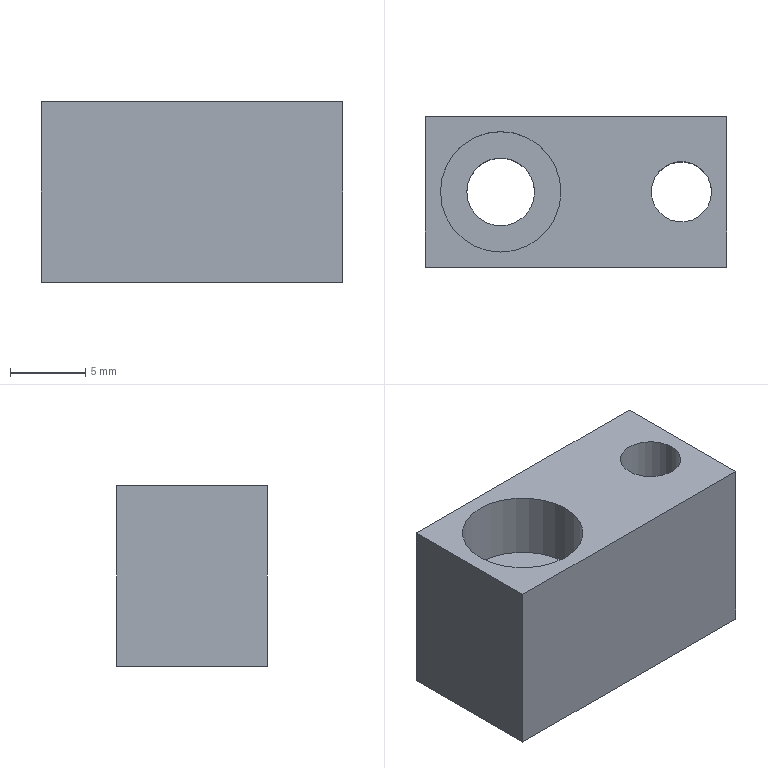Part | NX | features BREP 1 | 1 solid | 10 faces | box 20 x 10 x 12 mm | volume 1907 mm3 | plane 7 | cylinder 3 | commonest cylinder face diameters 4 x1 4.5 x1 8 x1
STEP:
#1=CARTESIAN_POINT('',(10.,-5.,0.));
#2=VERTEX_POINT('',#1);
#3=CARTESIAN_POINT('',(10.,5.,0.));
#4=VERTEX_POINT('',#3);
#5=CARTESIAN_POINT('',(10.,5.,0.));
#6=DIRECTION('',(0.,1.,0.));
#7=VECTOR('',#6,1000.);
#8=LINE('',#5,#7);
#9=EDGE_CURVE('',#2,#4,#8,.T.);
#10=ORIENTED_EDGE('',*,*,#9,.F.);
#11=CARTESIAN_POINT('',(10.,-5.,-12.));
#12=VERTEX_POINT('',#11);
#13=CARTESIAN_POINT('',(10.,-5.,-12.));
#14=DIRECTION('',(0.,0.,1.));
#15=VECTOR('',#14,1000.);
#16=LINE('',#13,#15);
#17=EDGE_CURVE('',#12,#2,#16,.T.);
#18=ORIENTED_EDGE('',*,*,#17,.F.);
#19=CARTESIAN_POINT('',(10.,5.,-12.));
#20=VERTEX_POINT('',#19);
#21=CARTESIAN_POINT('',(10.,5.,-12.));
#22=DIRECTION('',(0.,1.,0.));
#23=VECTOR('',#22,1000.);
#24=LINE('',#21,#23);
#25=EDGE_CURVE('',#12,#20,#24,.T.);
#26=ORIENTED_EDGE('',*,*,#25,.T.);
#27=CARTESIAN_POINT('',(10.,5.,-12.));
#28=DIRECTION('',(0.,0.,1.));
#29=VECTOR('',#28,1000.);
#30=LINE('',#27,#29);
#31=EDGE_CURVE('',#20,#4,#30,.T.);
#32=ORIENTED_EDGE('',*,*,#31,.T.);
#33=EDGE_LOOP('',(#10,#18,#26,#32));
#34=FACE_BOUND('',#33,.T.);
#35=CARTESIAN_POINT('',(10.,5.,-12.));
#36=DIRECTION('',(-1.,0.,0.));
#37=DIRECTION('',(0.,0.,1.));
#38=AXIS2_PLACEMENT_3D('',#35,#36,#37);
#39=PLANE('',#38);
#40=ADVANCED_FACE('',(#34),#39,.F.);
#41=CARTESIAN_POINT('',(-10.,5.,0.));
#42=VERTEX_POINT('',#41);
#43=CARTESIAN_POINT('',(-10.,5.,0.));
#44=DIRECTION('',(-1.,0.,0.));
#45=VECTOR('',#44,1000.);
#46=LINE('',#43,#45);
#47=EDGE_CURVE('',#4,#42,#46,.T.);
#48=ORIENTED_EDGE('',*,*,#47,.F.);
#49=ORIENTED_EDGE('',*,*,#31,.F.);
#50=CARTESIAN_POINT('',(-10.,5.,-12.));
#51=VERTEX_POINT('',#50);
#52=CARTESIAN_POINT('',(-10.,5.,-12.));
#53=DIRECTION('',(-1.,0.,0.));
#54=VECTOR('',#53,1000.);
#55=LINE('',#52,#54);
#56=EDGE_CURVE('',#20,#51,#55,.T.);
#57=ORIENTED_EDGE('',*,*,#56,.T.);
#58=CARTESIAN_POINT('',(-10.,5.,-12.));
#59=DIRECTION('',(0.,0.,1.));
#60=VECTOR('',#59,1000.);
#61=LINE('',#58,#60);
#62=EDGE_CURVE('',#51,#42,#61,.T.);
#63=ORIENTED_EDGE('',*,*,#62,.T.);
#64=EDGE_LOOP('',(#48,#49,#57,#63));
#65=FACE_BOUND('',#64,.T.);
#66=CARTESIAN_POINT('',(-10.,5.,-12.));
#67=DIRECTION('',(0.,-1.,0.));
#68=DIRECTION('',(0.,0.,-1.));
#69=AXIS2_PLACEMENT_3D('',#66,#67,#68);
#70=PLANE('',#69);
#71=ADVANCED_FACE('',(#65),#70,.F.);
#72=CARTESIAN_POINT('',(-10.,-5.,0.));
#73=VERTEX_POINT('',#72);
#74=CARTESIAN_POINT('',(-10.,5.,0.));
#75=DIRECTION('',(0.,-1.,0.));
#76=VECTOR('',#75,1000.);
#77=LINE('',#74,#76);
#78=EDGE_CURVE('',#42,#73,#77,.T.);
#79=ORIENTED_EDGE('',*,*,#78,.F.);
#80=ORIENTED_EDGE('',*,*,#62,.F.);
#81=CARTESIAN_POINT('',(-10.,-5.,-12.));
#82=VERTEX_POINT('',#81);
#83=CARTESIAN_POINT('',(-10.,5.,-12.));
#84=DIRECTION('',(0.,-1.,0.));
#85=VECTOR('',#84,1000.);
#86=LINE('',#83,#85);
#87=EDGE_CURVE('',#51,#82,#86,.T.);
#88=ORIENTED_EDGE('',*,*,#87,.T.);
#89=CARTESIAN_POINT('',(-10.,-5.,-12.));
#90=DIRECTION('',(0.,0.,1.));
#91=VECTOR('',#90,1000.);
#92=LINE('',#89,#91);
#93=EDGE_CURVE('',#82,#73,#92,.T.);
#94=ORIENTED_EDGE('',*,*,#93,.T.);
#95=EDGE_LOOP('',(#79,#80,#88,#94));
#96=FACE_BOUND('',#95,.T.);
#97=CARTESIAN_POINT('',(-10.,5.,-12.));
#98=DIRECTION('',(1.,0.,0.));
#99=DIRECTION('',(0.,0.,-1.));
#100=AXIS2_PLACEMENT_3D('',#97,#98,#99);
#101=PLANE('',#100);
#102=ADVANCED_FACE('',(#96),#101,.F.);
#103=CARTESIAN_POINT('',(-10.,-5.,0.));
#104=DIRECTION('',(1.,0.,0.));
#105=VECTOR('',#104,1000.);
#106=LINE('',#103,#105);
#107=EDGE_CURVE('',#73,#2,#106,.T.);
#108=ORIENTED_EDGE('',*,*,#107,.F.);
#109=ORIENTED_EDGE('',*,*,#93,.F.);
#110=CARTESIAN_POINT('',(-10.,-5.,-12.));
#111=DIRECTION('',(1.,0.,0.));
#112=VECTOR('',#111,1000.);
#113=LINE('',#110,#112);
#114=EDGE_CURVE('',#82,#12,#113,.T.);
#115=ORIENTED_EDGE('',*,*,#114,.T.);
#116=ORIENTED_EDGE('',*,*,#17,.T.);
#117=EDGE_LOOP('',(#108,#109,#115,#116));
#118=FACE_BOUND('',#117,.T.);
#119=CARTESIAN_POINT('',(-10.,-5.,-12.));
#120=DIRECTION('',(0.,1.,0.));
#121=DIRECTION('',(0.,0.,1.));
#122=AXIS2_PLACEMENT_3D('',#119,#120,#121);
#123=PLANE('',#122);
#124=ADVANCED_FACE('',(#118),#123,.F.);
#125=CARTESIAN_POINT('',(-7.25,0.,-12.));
#126=VERTEX_POINT('',#125);
#127=CARTESIAN_POINT('',(-5.,0.,-12.));
#128=DIRECTION('',(0.,0.,-1.));
#129=DIRECTION('',(-1.,0.,0.));
#130=AXIS2_PLACEMENT_3D('',#127,#128,#129);
#131=CIRCLE('',#130,2.25);
#132=EDGE_CURVE('',#126,#126,#131,.T.);
#133=ORIENTED_EDGE('',*,*,#132,.F.);
#134=EDGE_LOOP('',(#133));
#135=FACE_BOUND('',#134,.T.);
#136=CARTESIAN_POINT('',(5.,0.,-12.));
#137=VERTEX_POINT('',#136);
#138=CARTESIAN_POINT('',(7.,0.,-12.));
#139=DIRECTION('',(0.,0.,-1.));
#140=DIRECTION('',(-1.,0.,0.));
#141=AXIS2_PLACEMENT_3D('',#138,#139,#140);
#142=CIRCLE('',#141,2.);
#143=EDGE_CURVE('',#137,#137,#142,.T.);
#144=ORIENTED_EDGE('',*,*,#143,.F.);
#145=EDGE_LOOP('',(#144));
#146=FACE_BOUND('',#145,.T.);
#147=ORIENTED_EDGE('',*,*,#25,.F.);
#148=ORIENTED_EDGE('',*,*,#114,.F.);
#149=ORIENTED_EDGE('',*,*,#87,.F.);
#150=ORIENTED_EDGE('',*,*,#56,.F.);
#151=EDGE_LOOP('',(#147,#148,#149,#150));
#152=FACE_BOUND('',#151,.T.);
#153=CARTESIAN_POINT('',(0.,0.,-12.));
#154=DIRECTION('',(0.,0.,-1.));
#155=DIRECTION('',(-1.,0.,0.));
#156=AXIS2_PLACEMENT_3D('',#153,#154,#155);
#157=PLANE('',#156);
#158=ADVANCED_FACE('',(#135,#146,#152),#157,.T.);
#159=CARTESIAN_POINT('',(-9.,0.,0.));
#160=VERTEX_POINT('',#159);
#161=CARTESIAN_POINT('',(-5.,0.,0.));
#162=DIRECTION('',(0.,0.,-1.));
#163=DIRECTION('',(-1.,0.,0.));
#164=AXIS2_PLACEMENT_3D('',#161,#162,#163);
#165=CIRCLE('',#164,4.);
#166=EDGE_CURVE('',#160,#160,#165,.T.);
#167=ORIENTED_EDGE('',*,*,#166,.T.);
#168=EDGE_LOOP('',(#167));
#169=FACE_BOUND('',#168,.T.);
#170=CARTESIAN_POINT('',(5.,0.,0.));
#171=VERTEX_POINT('',#170);
#172=CARTESIAN_POINT('',(7.,0.,0.));
#173=DIRECTION('',(0.,0.,-1.));
#174=DIRECTION('',(-1.,0.,0.));
#175=AXIS2_PLACEMENT_3D('',#172,#173,#174);
#176=CIRCLE('',#175,2.);
#177=EDGE_CURVE('',#171,#171,#176,.T.);
#178=ORIENTED_EDGE('',*,*,#177,.T.);
#179=EDGE_LOOP('',(#178));
#180=FACE_BOUND('',#179,.T.);
#181=ORIENTED_EDGE('',*,*,#9,.T.);
#182=ORIENTED_EDGE('',*,*,#47,.T.);
#183=ORIENTED_EDGE('',*,*,#78,.T.);
#184=ORIENTED_EDGE('',*,*,#107,.T.);
#185=EDGE_LOOP('',(#181,#182,#183,#184));
#186=FACE_BOUND('',#185,.T.);
#187=CARTESIAN_POINT('',(0.,0.,0.));
#188=DIRECTION('',(0.,0.,-1.));
#189=DIRECTION('',(-1.,0.,0.));
#190=AXIS2_PLACEMENT_3D('',#187,#188,#189);
#191=PLANE('',#190);
#192=ADVANCED_FACE('',(#169,#180,#186),#191,.F.);
#193=ORIENTED_EDGE('',*,*,#143,.T.);
#194=EDGE_LOOP('',(#193));
#195=FACE_BOUND('',#194,.T.);
#196=ORIENTED_EDGE('',*,*,#177,.F.);
#197=EDGE_LOOP('',(#196));
#198=FACE_BOUND('',#197,.T.);
#199=CARTESIAN_POINT('',(7.,0.,0.));
#200=DIRECTION('',(0.,0.,1.));
#201=DIRECTION('',(1.,0.,0.));
#202=AXIS2_PLACEMENT_3D('',#199,#200,#201);
#203=CYLINDRICAL_SURFACE('',#202,2.);
#204=ADVANCED_FACE('',(#195,#198),#203,.F.);
#205=ORIENTED_EDGE('',*,*,#132,.T.);
#206=EDGE_LOOP('',(#205));
#207=FACE_BOUND('',#206,.T.);
#208=CARTESIAN_POINT('',(-7.25,0.,-4.4));
#209=VERTEX_POINT('',#208);
#210=CARTESIAN_POINT('',(-5.,0.,-4.4));
#211=DIRECTION('',(0.,0.,-1.));
#212=DIRECTION('',(-1.,0.,0.));
#213=AXIS2_PLACEMENT_3D('',#210,#211,#212);
#214=CIRCLE('',#213,2.25);
#215=EDGE_CURVE('',#209,#209,#214,.T.);
#216=ORIENTED_EDGE('',*,*,#215,.F.);
#217=EDGE_LOOP('',(#216));
#218=FACE_BOUND('',#217,.T.);
#219=CARTESIAN_POINT('',(-5.,0.,0.));
#220=DIRECTION('',(0.,0.,1.));
#221=DIRECTION('',(1.,0.,0.));
#222=AXIS2_PLACEMENT_3D('',#219,#220,#221);
#223=CYLINDRICAL_SURFACE('',#222,2.25);
#224=ADVANCED_FACE('',(#207,#218),#223,.F.);
#225=ORIENTED_EDGE('',*,*,#215,.T.);
#226=EDGE_LOOP('',(#225));
#227=FACE_BOUND('',#226,.T.);
#228=CARTESIAN_POINT('',(-9.,0.,-4.4));
#229=VERTEX_POINT('',#228);
#230=CARTESIAN_POINT('',(-5.,0.,-4.4));
#231=DIRECTION('',(0.,0.,-1.));
#232=DIRECTION('',(-1.,0.,0.));
#233=AXIS2_PLACEMENT_3D('',#230,#231,#232);
#234=CIRCLE('',#233,4.);
#235=EDGE_CURVE('',#229,#229,#234,.T.);
#236=ORIENTED_EDGE('',*,*,#235,.F.);
#237=EDGE_LOOP('',(#236));
#238=FACE_BOUND('',#237,.T.);
#239=CARTESIAN_POINT('',(-2.75,0.,-4.4));
#240=DIRECTION('',(0.,0.,-1.));
#241=DIRECTION('',(-1.,0.,0.));
#242=AXIS2_PLACEMENT_3D('',#239,#240,#241);
#243=PLANE('',#242);
#244=ADVANCED_FACE('',(#227,#238),#243,.F.);
#245=ORIENTED_EDGE('',*,*,#235,.T.);
#246=EDGE_LOOP('',(#245));
#247=FACE_BOUND('',#246,.T.);
#248=ORIENTED_EDGE('',*,*,#166,.F.);
#249=EDGE_LOOP('',(#248));
#250=FACE_BOUND('',#249,.T.);
#251=CARTESIAN_POINT('',(-5.,0.,0.));
#252=DIRECTION('',(0.,0.,1.));
#253=DIRECTION('',(1.,0.,0.));
#254=AXIS2_PLACEMENT_3D('',#251,#252,#253);
#255=CYLINDRICAL_SURFACE('',#254,4.);
#256=ADVANCED_FACE('',(#247,#250),#255,.F.);
#257=CLOSED_SHELL('',(#40,#71,#102,#124,#158,#192,#204,#224,#244,#256));
#258=MANIFOLD_SOLID_BREP('',#257);
#259=(LENGTH_UNIT()NAMED_UNIT(*)SI_UNIT(.MILLI.,.METRE.));
#260=UNCERTAINTY_MEASURE_WITH_UNIT(LENGTH_MEASURE(0.00001),#259,'','');
#261=(NAMED_UNIT(*)PLANE_ANGLE_UNIT()SI_UNIT($,.RADIAN.));
#262=(NAMED_UNIT(*)SI_UNIT($,.STERADIAN.)SOLID_ANGLE_UNIT());
#263=(GEOMETRIC_REPRESENTATION_CONTEXT(3)GLOBAL_UNCERTAINTY_ASSIGNED_CONTEXT((#260))GLOBAL_UNIT_ASSIGNED_CONTEXT((#259,#261,#262))REPRESENTATION_CONTEXT('',''));
#264=ADVANCED_BREP_SHAPE_REPRESENTATION('',(#258),#263);